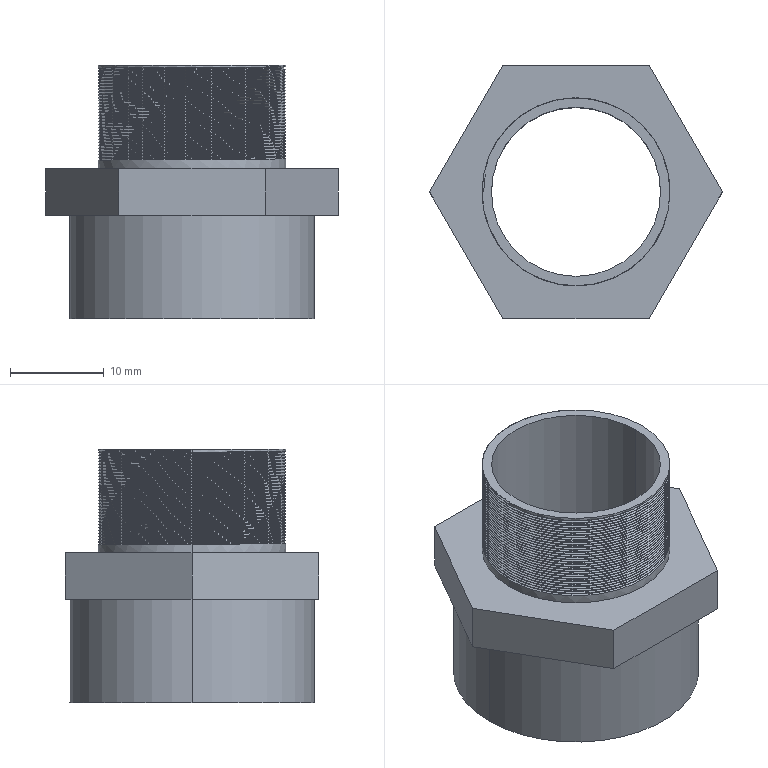Part | SolidWorks | features ICE 3, Extrusion 1, SweepThread 1 | 1 solid | 83 faces | box 31.177 x 27 x 27 mm | volume 5569 mm3 | cylinder 68 | plane 12 | spline 3 | commonest cylinder face diameters 20 x64 18 x2 26.1 x2